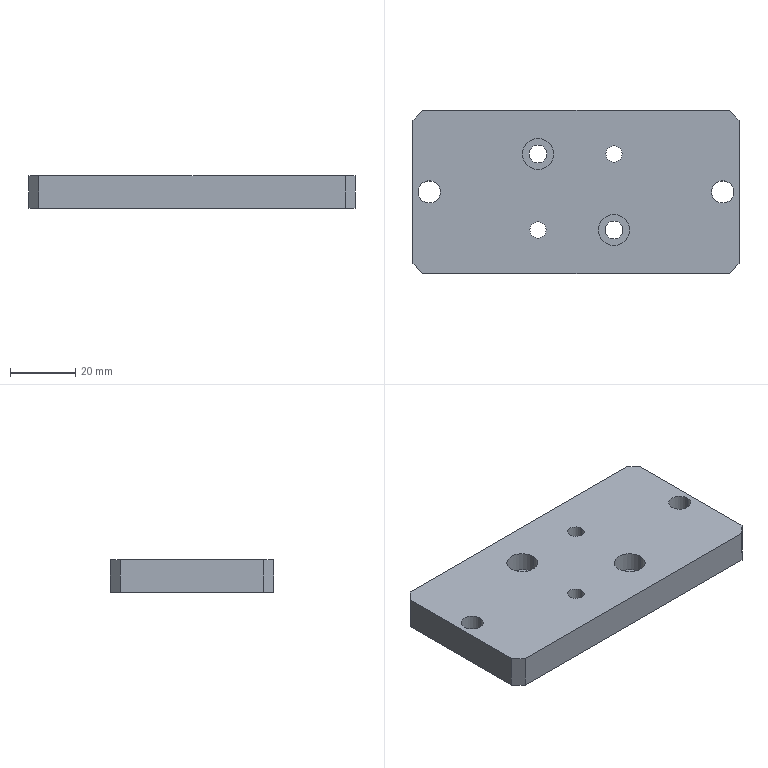Part | STEP file | PN_0002 top plate Default | 1 solid | 28 faces | box 100 x 50 x 10 mm | volume 47660 mm3 | cylinder 16 | plane 12 | commonest cylinder face diameters 5 x4 5.5 x4 6.8 x4 9.5 x4
STEP:
#1=CARTESIAN_POINT('',(-48.4,0.,0.));
#2=VERTEX_POINT('',#1);
#3=CARTESIAN_POINT('',(-41.6,0.,0.));
#4=VERTEX_POINT('',#3);
#5=CARTESIAN_POINT('',(-45.,0.,0.));
#6=DIRECTION('',(0.,0.,1.));
#7=DIRECTION('',(1.,0.,0.));
#8=AXIS2_PLACEMENT_3D('',#5,#6,#7);
#9=CIRCLE('',#8,3.4);
#10=EDGE_CURVE('',#2,#4,#9,.T.);
#11=ORIENTED_EDGE('',*,*,#10,.F.);
#12=CARTESIAN_POINT('',(-48.4,0.,10.));
#13=VERTEX_POINT('',#12);
#14=CARTESIAN_POINT('',(-48.4,0.,10.));
#15=DIRECTION('',(0.,0.,1.));
#16=VECTOR('',#15,1000.);
#17=LINE('',#14,#16);
#18=EDGE_CURVE('',#2,#13,#17,.T.);
#19=ORIENTED_EDGE('',*,*,#18,.T.);
#20=CARTESIAN_POINT('',(-41.6,0.,10.));
#21=VERTEX_POINT('',#20);
#22=CARTESIAN_POINT('',(-45.,0.,10.));
#23=DIRECTION('',(0.,0.,1.));
#24=DIRECTION('',(1.,0.,0.));
#25=AXIS2_PLACEMENT_3D('',#22,#23,#24);
#26=CIRCLE('',#25,3.4);
#27=EDGE_CURVE('',#13,#21,#26,.T.);
#28=ORIENTED_EDGE('',*,*,#27,.T.);
#29=CARTESIAN_POINT('',(-41.6,0.,10.));
#30=DIRECTION('',(0.,0.,1.));
#31=VECTOR('',#30,1000.);
#32=LINE('',#29,#31);
#33=EDGE_CURVE('',#4,#21,#32,.T.);
#34=ORIENTED_EDGE('',*,*,#33,.F.);
#35=EDGE_LOOP('',(#11,#19,#28,#34));
#36=FACE_OUTER_BOUND('',#35,.T.);
#37=CARTESIAN_POINT('',(-45.,0.,10.));
#38=DIRECTION('',(0.,0.,1.));
#39=DIRECTION('',(1.,0.,0.));
#40=AXIS2_PLACEMENT_3D('',#37,#38,#39);
#41=CYLINDRICAL_SURFACE('',#40,3.4);
#42=ADVANCED_FACE('',(#36),#41,.F.);
#43=CARTESIAN_POINT('',(41.6,0.,0.));
#44=VERTEX_POINT('',#43);
#45=CARTESIAN_POINT('',(48.4,0.,0.));
#46=VERTEX_POINT('',#45);
#47=CARTESIAN_POINT('',(45.,0.,0.));
#48=DIRECTION('',(0.,0.,1.));
#49=DIRECTION('',(1.,0.,0.));
#50=AXIS2_PLACEMENT_3D('',#47,#48,#49);
#51=CIRCLE('',#50,3.4);
#52=EDGE_CURVE('',#44,#46,#51,.T.);
#53=ORIENTED_EDGE('',*,*,#52,.F.);
#54=CARTESIAN_POINT('',(41.6,0.,10.));
#55=VERTEX_POINT('',#54);
#56=CARTESIAN_POINT('',(41.6,0.,10.));
#57=DIRECTION('',(0.,0.,1.));
#58=VECTOR('',#57,1000.);
#59=LINE('',#56,#58);
#60=EDGE_CURVE('',#44,#55,#59,.T.);
#61=ORIENTED_EDGE('',*,*,#60,.T.);
#62=CARTESIAN_POINT('',(48.4,0.,10.));
#63=VERTEX_POINT('',#62);
#64=CARTESIAN_POINT('',(45.,0.,10.));
#65=DIRECTION('',(0.,0.,1.));
#66=DIRECTION('',(1.,0.,0.));
#67=AXIS2_PLACEMENT_3D('',#64,#65,#66);
#68=CIRCLE('',#67,3.4);
#69=EDGE_CURVE('',#55,#63,#68,.T.);
#70=ORIENTED_EDGE('',*,*,#69,.T.);
#71=CARTESIAN_POINT('',(48.4,0.,10.));
#72=DIRECTION('',(0.,0.,1.));
#73=VECTOR('',#72,1000.);
#74=LINE('',#71,#73);
#75=EDGE_CURVE('',#46,#63,#74,.T.);
#76=ORIENTED_EDGE('',*,*,#75,.F.);
#77=EDGE_LOOP('',(#53,#61,#70,#76));
#78=FACE_OUTER_BOUND('',#77,.T.);
#79=CARTESIAN_POINT('',(45.,0.,10.));
#80=DIRECTION('',(0.,0.,1.));
#81=DIRECTION('',(1.,0.,0.));
#82=AXIS2_PLACEMENT_3D('',#79,#80,#81);
#83=CYLINDRICAL_SURFACE('',#82,3.4);
#84=ADVANCED_FACE('',(#78),#83,.F.);
#85=CARTESIAN_POINT('',(9.15,11.65,0.));
#86=VERTEX_POINT('',#85);
#87=CARTESIAN_POINT('',(14.15,11.65,0.));
#88=VERTEX_POINT('',#87);
#89=CARTESIAN_POINT('',(11.65,11.65,0.));
#90=DIRECTION('',(0.,0.,1.));
#91=DIRECTION('',(1.,0.,0.));
#92=AXIS2_PLACEMENT_3D('',#89,#90,#91);
#93=CIRCLE('',#92,2.5);
#94=EDGE_CURVE('',#86,#88,#93,.T.);
#95=ORIENTED_EDGE('',*,*,#94,.F.);
#96=CARTESIAN_POINT('',(9.15,11.65,10.));
#97=VERTEX_POINT('',#96);
#98=CARTESIAN_POINT('',(9.15,11.65,10.));
#99=DIRECTION('',(0.,0.,1.));
#100=VECTOR('',#99,1000.);
#101=LINE('',#98,#100);
#102=EDGE_CURVE('',#86,#97,#101,.T.);
#103=ORIENTED_EDGE('',*,*,#102,.T.);
#104=CARTESIAN_POINT('',(14.15,11.65,10.));
#105=VERTEX_POINT('',#104);
#106=CARTESIAN_POINT('',(11.65,11.65,10.));
#107=DIRECTION('',(0.,0.,1.));
#108=DIRECTION('',(1.,0.,0.));
#109=AXIS2_PLACEMENT_3D('',#106,#107,#108);
#110=CIRCLE('',#109,2.5);
#111=EDGE_CURVE('',#97,#105,#110,.T.);
#112=ORIENTED_EDGE('',*,*,#111,.T.);
#113=CARTESIAN_POINT('',(14.15,11.65,10.));
#114=DIRECTION('',(0.,0.,1.));
#115=VECTOR('',#114,1000.);
#116=LINE('',#113,#115);
#117=EDGE_CURVE('',#88,#105,#116,.T.);
#118=ORIENTED_EDGE('',*,*,#117,.F.);
#119=EDGE_LOOP('',(#95,#103,#112,#118));
#120=FACE_OUTER_BOUND('',#119,.T.);
#121=CARTESIAN_POINT('',(11.65,11.65,10.));
#122=DIRECTION('',(0.,0.,1.));
#123=DIRECTION('',(1.,0.,0.));
#124=AXIS2_PLACEMENT_3D('',#121,#122,#123);
#125=CYLINDRICAL_SURFACE('',#124,2.5);
#126=ADVANCED_FACE('',(#120),#125,.F.);
#127=CARTESIAN_POINT('',(-14.15,-11.65,0.));
#128=VERTEX_POINT('',#127);
#129=CARTESIAN_POINT('',(-9.15,-11.65,0.));
#130=VERTEX_POINT('',#129);
#131=CARTESIAN_POINT('',(-11.65,-11.65,0.));
#132=DIRECTION('',(0.,0.,1.));
#133=DIRECTION('',(1.,0.,0.));
#134=AXIS2_PLACEMENT_3D('',#131,#132,#133);
#135=CIRCLE('',#134,2.5);
#136=EDGE_CURVE('',#128,#130,#135,.T.);
#137=ORIENTED_EDGE('',*,*,#136,.F.);
#138=CARTESIAN_POINT('',(-14.15,-11.65,10.));
#139=VERTEX_POINT('',#138);
#140=CARTESIAN_POINT('',(-14.15,-11.65,10.));
#141=DIRECTION('',(0.,0.,1.));
#142=VECTOR('',#141,1000.);
#143=LINE('',#140,#142);
#144=EDGE_CURVE('',#128,#139,#143,.T.);
#145=ORIENTED_EDGE('',*,*,#144,.T.);
#146=CARTESIAN_POINT('',(-9.15,-11.65,10.));
#147=VERTEX_POINT('',#146);
#148=CARTESIAN_POINT('',(-11.65,-11.65,10.));
#149=DIRECTION('',(0.,0.,1.));
#150=DIRECTION('',(1.,0.,0.));
#151=AXIS2_PLACEMENT_3D('',#148,#149,#150);
#152=CIRCLE('',#151,2.5);
#153=EDGE_CURVE('',#139,#147,#152,.T.);
#154=ORIENTED_EDGE('',*,*,#153,.T.);
#155=CARTESIAN_POINT('',(-9.15,-11.65,10.));
#156=DIRECTION('',(0.,0.,1.));
#157=VECTOR('',#156,1000.);
#158=LINE('',#155,#157);
#159=EDGE_CURVE('',#130,#147,#158,.T.);
#160=ORIENTED_EDGE('',*,*,#159,.F.);
#161=EDGE_LOOP('',(#137,#145,#154,#160));
#162=FACE_OUTER_BOUND('',#161,.T.);
#163=CARTESIAN_POINT('',(-11.65,-11.65,10.));
#164=DIRECTION('',(0.,0.,1.));
#165=DIRECTION('',(1.,0.,0.));
#166=AXIS2_PLACEMENT_3D('',#163,#164,#165);
#167=CYLINDRICAL_SURFACE('',#166,2.5);
#168=ADVANCED_FACE('',(#162),#167,.F.);
#169=CARTESIAN_POINT('',(6.9,-11.65,4.));
#170=VERTEX_POINT('',#169);
#171=CARTESIAN_POINT('',(16.4,-11.65,4.));
#172=VERTEX_POINT('',#171);
#173=CARTESIAN_POINT('',(11.65,-11.65,4.));
#174=DIRECTION('',(0.,0.,1.));
#175=DIRECTION('',(1.,0.,0.));
#176=AXIS2_PLACEMENT_3D('',#173,#174,#175);
#177=CIRCLE('',#176,4.75);
#178=EDGE_CURVE('',#170,#172,#177,.T.);
#179=ORIENTED_EDGE('',*,*,#178,.F.);
#180=CARTESIAN_POINT('',(6.9,-11.65,10.));
#181=VERTEX_POINT('',#180);
#182=CARTESIAN_POINT('',(6.9,-11.65,10.));
#183=DIRECTION('',(0.,0.,1.));
#184=VECTOR('',#183,1000.);
#185=LINE('',#182,#184);
#186=EDGE_CURVE('',#170,#181,#185,.T.);
#187=ORIENTED_EDGE('',*,*,#186,.T.);
#188=CARTESIAN_POINT('',(16.4,-11.65,10.));
#189=VERTEX_POINT('',#188);
#190=CARTESIAN_POINT('',(11.65,-11.65,10.));
#191=DIRECTION('',(0.,0.,1.));
#192=DIRECTION('',(1.,0.,0.));
#193=AXIS2_PLACEMENT_3D('',#190,#191,#192);
#194=CIRCLE('',#193,4.75);
#195=EDGE_CURVE('',#181,#189,#194,.T.);
#196=ORIENTED_EDGE('',*,*,#195,.T.);
#197=CARTESIAN_POINT('',(16.4,-11.65,10.));
#198=DIRECTION('',(0.,0.,1.));
#199=VECTOR('',#198,1000.);
#200=LINE('',#197,#199);
#201=EDGE_CURVE('',#172,#189,#200,.T.);
#202=ORIENTED_EDGE('',*,*,#201,.F.);
#203=EDGE_LOOP('',(#179,#187,#196,#202));
#204=FACE_OUTER_BOUND('',#203,.T.);
#205=CARTESIAN_POINT('',(11.65,-11.65,10.));
#206=DIRECTION('',(0.,0.,1.));
#207=DIRECTION('',(1.,0.,0.));
#208=AXIS2_PLACEMENT_3D('',#205,#206,#207);
#209=CYLINDRICAL_SURFACE('',#208,4.75);
#210=ADVANCED_FACE('',(#204),#209,.F.);
#211=CARTESIAN_POINT('',(8.9,-11.65,0.));
#212=VERTEX_POINT('',#211);
#213=CARTESIAN_POINT('',(14.4,-11.65,0.));
#214=VERTEX_POINT('',#213);
#215=CARTESIAN_POINT('',(11.65,-11.65,0.));
#216=DIRECTION('',(0.,0.,1.));
#217=DIRECTION('',(1.,0.,0.));
#218=AXIS2_PLACEMENT_3D('',#215,#216,#217);
#219=CIRCLE('',#218,2.75);
#220=EDGE_CURVE('',#212,#214,#219,.T.);
#221=ORIENTED_EDGE('',*,*,#220,.F.);
#222=CARTESIAN_POINT('',(8.9,-11.65,4.));
#223=VERTEX_POINT('',#222);
#224=CARTESIAN_POINT('',(8.9,-11.65,10.));
#225=DIRECTION('',(0.,0.,1.));
#226=VECTOR('',#225,1000.);
#227=LINE('',#224,#226);
#228=EDGE_CURVE('',#212,#223,#227,.T.);
#229=ORIENTED_EDGE('',*,*,#228,.T.);
#230=CARTESIAN_POINT('',(14.4,-11.65,4.));
#231=VERTEX_POINT('',#230);
#232=CARTESIAN_POINT('',(11.65,-11.65,4.));
#233=DIRECTION('',(0.,0.,1.));
#234=DIRECTION('',(1.,0.,0.));
#235=AXIS2_PLACEMENT_3D('',#232,#233,#234);
#236=CIRCLE('',#235,2.75);
#237=EDGE_CURVE('',#223,#231,#236,.T.);
#238=ORIENTED_EDGE('',*,*,#237,.T.);
#239=CARTESIAN_POINT('',(14.4,-11.65,10.));
#240=DIRECTION('',(0.,0.,1.));
#241=VECTOR('',#240,1000.);
#242=LINE('',#239,#241);
#243=EDGE_CURVE('',#214,#231,#242,.T.);
#244=ORIENTED_EDGE('',*,*,#243,.F.);
#245=EDGE_LOOP('',(#221,#229,#238,#244));
#246=FACE_OUTER_BOUND('',#245,.T.);
#247=CARTESIAN_POINT('',(11.65,-11.65,10.));
#248=DIRECTION('',(0.,0.,1.));
#249=DIRECTION('',(1.,0.,0.));
#250=AXIS2_PLACEMENT_3D('',#247,#248,#249);
#251=CYLINDRICAL_SURFACE('',#250,2.75);
#252=ADVANCED_FACE('',(#246),#251,.F.);
#253=CARTESIAN_POINT('',(-16.4,11.65,4.));
#254=VERTEX_POINT('',#253);
#255=CARTESIAN_POINT('',(-6.9,11.65,4.));
#256=VERTEX_POINT('',#255);
#257=CARTESIAN_POINT('',(-11.65,11.65,4.));
#258=DIRECTION('',(0.,0.,1.));
#259=DIRECTION('',(1.,0.,0.));
#260=AXIS2_PLACEMENT_3D('',#257,#258,#259);
#261=CIRCLE('',#260,4.75);
#262=EDGE_CURVE('',#254,#256,#261,.T.);
#263=ORIENTED_EDGE('',*,*,#262,.F.);
#264=CARTESIAN_POINT('',(-16.4,11.65,10.));
#265=VERTEX_POINT('',#264);
#266=CARTESIAN_POINT('',(-16.4,11.65,10.));
#267=DIRECTION('',(0.,0.,1.));
#268=VECTOR('',#267,1000.);
#269=LINE('',#266,#268);
#270=EDGE_CURVE('',#254,#265,#269,.T.);
#271=ORIENTED_EDGE('',*,*,#270,.T.);
#272=CARTESIAN_POINT('',(-6.9,11.65,10.));
#273=VERTEX_POINT('',#272);
#274=CARTESIAN_POINT('',(-11.65,11.65,10.));
#275=DIRECTION('',(0.,0.,1.));
#276=DIRECTION('',(1.,0.,0.));
#277=AXIS2_PLACEMENT_3D('',#274,#275,#276);
#278=CIRCLE('',#277,4.75);
#279=EDGE_CURVE('',#265,#273,#278,.T.);
#280=ORIENTED_EDGE('',*,*,#279,.T.);
#281=CARTESIAN_POINT('',(-6.9,11.65,10.));
#282=DIRECTION('',(0.,0.,1.));
#283=VECTOR('',#282,1000.);
#284=LINE('',#281,#283);
#285=EDGE_CURVE('',#256,#273,#284,.T.);
#286=ORIENTED_EDGE('',*,*,#285,.F.);
#287=EDGE_LOOP('',(#263,#271,#280,#286));
#288=FACE_OUTER_BOUND('',#287,.T.);
#289=CARTESIAN_POINT('',(-11.65,11.65,10.));
#290=DIRECTION('',(0.,0.,1.));
#291=DIRECTION('',(1.,0.,0.));
#292=AXIS2_PLACEMENT_3D('',#289,#290,#291);
#293=CYLINDRICAL_SURFACE('',#292,4.75);
#294=ADVANCED_FACE('',(#288),#293,.F.);
#295=CARTESIAN_POINT('',(-14.4,11.65,0.));
#296=VERTEX_POINT('',#295);
#297=CARTESIAN_POINT('',(-8.9,11.65,0.));
#298=VERTEX_POINT('',#297);
#299=CARTESIAN_POINT('',(-11.65,11.65,0.));
#300=DIRECTION('',(0.,0.,1.));
#301=DIRECTION('',(1.,0.,0.));
#302=AXIS2_PLACEMENT_3D('',#299,#300,#301);
#303=CIRCLE('',#302,2.75);
#304=EDGE_CURVE('',#296,#298,#303,.T.);
#305=ORIENTED_EDGE('',*,*,#304,.F.);
#306=CARTESIAN_POINT('',(-14.4,11.65,4.));
#307=VERTEX_POINT('',#306);
#308=CARTESIAN_POINT('',(-14.4,11.65,10.));
#309=DIRECTION('',(0.,0.,1.));
#310=VECTOR('',#309,1000.);
#311=LINE('',#308,#310);
#312=EDGE_CURVE('',#296,#307,#311,.T.);
#313=ORIENTED_EDGE('',*,*,#312,.T.);
#314=CARTESIAN_POINT('',(-8.9,11.65,4.));
#315=VERTEX_POINT('',#314);
#316=CARTESIAN_POINT('',(-11.65,11.65,4.));
#317=DIRECTION('',(0.,0.,1.));
#318=DIRECTION('',(1.,0.,0.));
#319=AXIS2_PLACEMENT_3D('',#316,#317,#318);
#320=CIRCLE('',#319,2.75);
#321=EDGE_CURVE('',#307,#315,#320,.T.);
#322=ORIENTED_EDGE('',*,*,#321,.T.);
#323=CARTESIAN_POINT('',(-8.9,11.65,10.));
#324=DIRECTION('',(0.,0.,1.));
#325=VECTOR('',#324,1000.);
#326=LINE('',#323,#325);
#327=EDGE_CURVE('',#298,#315,#326,.T.);
#328=ORIENTED_EDGE('',*,*,#327,.F.);
#329=EDGE_LOOP('',(#305,#313,#322,#328));
#330=FACE_OUTER_BOUND('',#329,.T.);
#331=CARTESIAN_POINT('',(-11.65,11.65,10.));
#332=DIRECTION('',(0.,0.,1.));
#333=DIRECTION('',(1.,0.,0.));
#334=AXIS2_PLACEMENT_3D('',#331,#332,#333);
#335=CYLINDRICAL_SURFACE('',#334,2.75);
#336=ADVANCED_FACE('',(#330),#335,.F.);
#337=CARTESIAN_POINT('',(50.,-22.,0.));
#338=VERTEX_POINT('',#337);
#339=CARTESIAN_POINT('',(50.,22.,0.));
#340=VERTEX_POINT('',#339);
#341=CARTESIAN_POINT('',(50.,25.,0.));
#342=DIRECTION('',(0.,1.,0.));
#343=VECTOR('',#342,1000.);
#344=LINE('',#341,#343);
#345=EDGE_CURVE('',#338,#340,#344,.T.);
#346=ORIENTED_EDGE('',*,*,#345,.T.);
#347=CARTESIAN_POINT('',(50.,22.,10.));
#348=VERTEX_POINT('',#347);
#349=CARTESIAN_POINT('',(50.,22.,10.));
#350=DIRECTION('',(0.,0.,1.));
#351=VECTOR('',#350,1000.);
#352=LINE('',#349,#351);
#353=EDGE_CURVE('',#340,#348,#352,.T.);
#354=ORIENTED_EDGE('',*,*,#353,.T.);
#355=CARTESIAN_POINT('',(50.,-22.,10.));
#356=VERTEX_POINT('',#355);
#357=CARTESIAN_POINT('',(50.,25.,10.));
#358=DIRECTION('',(0.,1.,0.));
#359=VECTOR('',#358,1000.);
#360=LINE('',#357,#359);
#361=EDGE_CURVE('',#356,#348,#360,.T.);
#362=ORIENTED_EDGE('',*,*,#361,.F.);
#363=CARTESIAN_POINT('',(50.,-22.,10.));
#364=DIRECTION('',(0.,0.,-1.));
#365=VECTOR('',#364,1000.);
#366=LINE('',#363,#365);
#367=EDGE_CURVE('',#356,#338,#366,.T.);
#368=ORIENTED_EDGE('',*,*,#367,.T.);
#369=EDGE_LOOP('',(#346,#354,#362,#368));
#370=FACE_OUTER_BOUND('',#369,.T.);
#371=CARTESIAN_POINT('',(50.,25.,10.));
#372=DIRECTION('',(-1.,0.,0.));
#373=DIRECTION('',(0.,-1.,0.));
#374=AXIS2_PLACEMENT_3D('',#371,#372,#373);
#375=PLANE('',#374);
#376=ADVANCED_FACE('',(#370),#375,.F.);
#377=CARTESIAN_POINT('',(47.,25.,0.));
#378=VERTEX_POINT('',#377);
#379=CARTESIAN_POINT('',(-47.,25.,0.));
#380=VERTEX_POINT('',#379);
#381=CARTESIAN_POINT('',(-50.,25.,0.));
#382=DIRECTION('',(-1.,0.,0.));
#383=VECTOR('',#382,1000.);
#384=LINE('',#381,#383);
#385=EDGE_CURVE('',#378,#380,#384,.T.);
#386=ORIENTED_EDGE('',*,*,#385,.T.);
#387=CARTESIAN_POINT('',(-47.,25.,10.));
#388=VERTEX_POINT('',#387);
#389=CARTESIAN_POINT('',(-47.,25.,10.));
#390=DIRECTION('',(0.,0.,1.));
#391=VECTOR('',#390,1000.);
#392=LINE('',#389,#391);
#393=EDGE_CURVE('',#380,#388,#392,.T.);
#394=ORIENTED_EDGE('',*,*,#393,.T.);
#395=CARTESIAN_POINT('',(47.,25.,10.));
#396=VERTEX_POINT('',#395);
#397=CARTESIAN_POINT('',(-50.,25.,10.));
#398=DIRECTION('',(-1.,0.,0.));
#399=VECTOR('',#398,1000.);
#400=LINE('',#397,#399);
#401=EDGE_CURVE('',#396,#388,#400,.T.);
#402=ORIENTED_EDGE('',*,*,#401,.F.);
#403=CARTESIAN_POINT('',(47.,25.,10.));
#404=DIRECTION('',(0.,0.,-1.));
#405=VECTOR('',#404,1000.);
#406=LINE('',#403,#405);
#407=EDGE_CURVE('',#396,#378,#406,.T.);
#408=ORIENTED_EDGE('',*,*,#407,.T.);
#409=EDGE_LOOP('',(#386,#394,#402,#408));
#410=FACE_OUTER_BOUND('',#409,.T.);
#411=CARTESIAN_POINT('',(-50.,25.,10.));
#412=DIRECTION('',(0.,-1.,0.));
#413=DIRECTION('',(0.,0.,-1.));
#414=AXIS2_PLACEMENT_3D('',#411,#412,#413);
#415=PLANE('',#414);
#416=ADVANCED_FACE('',(#410),#415,.F.);
#417=CARTESIAN_POINT('',(-50.,22.,10.));
#418=VERTEX_POINT('',#417);
#419=CARTESIAN_POINT('',(-50.,-22.,10.));
#420=VERTEX_POINT('',#419);
#421=CARTESIAN_POINT('',(-50.,25.,10.));
#422=DIRECTION('',(0.,-1.,0.));
#423=VECTOR('',#422,1000.);
#424=LINE('',#421,#423);
#425=EDGE_CURVE('',#418,#420,#424,.T.);
#426=ORIENTED_EDGE('',*,*,#425,.F.);
#427=CARTESIAN_POINT('',(-50.,22.,0.));
#428=VERTEX_POINT('',#427);
#429=CARTESIAN_POINT('',(-50.,22.,10.));
#430=DIRECTION('',(0.,0.,-1.));
#431=VECTOR('',#430,1000.);
#432=LINE('',#429,#431);
#433=EDGE_CURVE('',#418,#428,#432,.T.);
#434=ORIENTED_EDGE('',*,*,#433,.T.);
#435=CARTESIAN_POINT('',(-50.,-22.,0.));
#436=VERTEX_POINT('',#435);
#437=CARTESIAN_POINT('',(-50.,25.,0.));
#438=DIRECTION('',(0.,-1.,0.));
#439=VECTOR('',#438,1000.);
#440=LINE('',#437,#439);
#441=EDGE_CURVE('',#428,#436,#440,.T.);
#442=ORIENTED_EDGE('',*,*,#441,.T.);
#443=CARTESIAN_POINT('',(-50.,-22.,10.));
#444=DIRECTION('',(0.,0.,1.));
#445=VECTOR('',#444,1000.);
#446=LINE('',#443,#445);
#447=EDGE_CURVE('',#436,#420,#446,.T.);
#448=ORIENTED_EDGE('',*,*,#447,.T.);
#449=EDGE_LOOP('',(#426,#434,#442,#448));
#450=FACE_OUTER_BOUND('',#449,.T.);
#451=CARTESIAN_POINT('',(-50.,25.,10.));
#452=DIRECTION('',(1.,0.,0.));
#453=DIRECTION('',(0.,1.,0.));
#454=AXIS2_PLACEMENT_3D('',#451,#452,#453);
#455=PLANE('',#454);
#456=ADVANCED_FACE('',(#450),#455,.F.);
#457=CARTESIAN_POINT('',(-47.,-25.,0.));
#458=VERTEX_POINT('',#457);
#459=CARTESIAN_POINT('',(47.,-25.,0.));
#460=VERTEX_POINT('',#459);
#461=CARTESIAN_POINT('',(-50.,-25.,0.));
#462=DIRECTION('',(1.,0.,0.));
#463=VECTOR('',#462,1000.);
#464=LINE('',#461,#463);
#465=EDGE_CURVE('',#458,#460,#464,.T.);
#466=ORIENTED_EDGE('',*,*,#465,.T.);
#467=CARTESIAN_POINT('',(47.,-25.,10.));
#468=VERTEX_POINT('',#467);
#469=CARTESIAN_POINT('',(47.,-25.,10.));
#470=DIRECTION('',(0.,0.,1.));
#471=VECTOR('',#470,1000.);
#472=LINE('',#469,#471);
#473=EDGE_CURVE('',#460,#468,#472,.T.);
#474=ORIENTED_EDGE('',*,*,#473,.T.);
#475=CARTESIAN_POINT('',(-47.,-25.,10.));
#476=VERTEX_POINT('',#475);
#477=CARTESIAN_POINT('',(-50.,-25.,10.));
#478=DIRECTION('',(1.,0.,0.));
#479=VECTOR('',#478,1000.);
#480=LINE('',#477,#479);
#481=EDGE_CURVE('',#476,#468,#480,.T.);
#482=ORIENTED_EDGE('',*,*,#481,.F.);
#483=CARTESIAN_POINT('',(-47.,-25.,10.));
#484=DIRECTION('',(0.,0.,-1.));
#485=VECTOR('',#484,1000.);
#486=LINE('',#483,#485);
#487=EDGE_CURVE('',#476,#458,#486,.T.);
#488=ORIENTED_EDGE('',*,*,#487,.T.);
#489=EDGE_LOOP('',(#466,#474,#482,#488));
#490=FACE_OUTER_BOUND('',#489,.T.);
#491=CARTESIAN_POINT('',(-50.,-25.,10.));
#492=DIRECTION('',(0.,1.,0.));
#493=DIRECTION('',(0.,0.,1.));
#494=AXIS2_PLACEMENT_3D('',#491,#492,#493);
#495=PLANE('',#494);
#496=ADVANCED_FACE('',(#490),#495,.F.);
#497=CARTESIAN_POINT('',(-45.,0.,10.));
#498=DIRECTION('',(0.,0.,1.));
#499=DIRECTION('',(1.,0.,0.));
#500=AXIS2_PLACEMENT_3D('',#497,#498,#499);
#501=CIRCLE('',#500,3.4);
#502=EDGE_CURVE('',#21,#13,#501,.T.);
#503=ORIENTED_EDGE('',*,*,#502,.F.);
#504=ORIENTED_EDGE('',*,*,#27,.F.);
#505=EDGE_LOOP('',(#503,#504));
#506=FACE_BOUND('',#505,.T.);
#507=CARTESIAN_POINT('',(45.,0.,10.));
#508=DIRECTION('',(0.,0.,1.));
#509=DIRECTION('',(1.,0.,0.));
#510=AXIS2_PLACEMENT_3D('',#507,#508,#509);
#511=CIRCLE('',#510,3.4);
#512=EDGE_CURVE('',#63,#55,#511,.T.);
#513=ORIENTED_EDGE('',*,*,#512,.F.);
#514=ORIENTED_EDGE('',*,*,#69,.F.);
#515=EDGE_LOOP('',(#513,#514));
#516=FACE_BOUND('',#515,.T.);
#517=CARTESIAN_POINT('',(11.65,11.65,10.));
#518=DIRECTION('',(0.,0.,1.));
#519=DIRECTION('',(1.,0.,0.));
#520=AXIS2_PLACEMENT_3D('',#517,#518,#519);
#521=CIRCLE('',#520,2.5);
#522=EDGE_CURVE('',#105,#97,#521,.T.);
#523=ORIENTED_EDGE('',*,*,#522,.F.);
#524=ORIENTED_EDGE('',*,*,#111,.F.);
#525=EDGE_LOOP('',(#523,#524));
#526=FACE_BOUND('',#525,.T.);
#527=CARTESIAN_POINT('',(-11.65,-11.65,10.));
#528=DIRECTION('',(0.,0.,1.));
#529=DIRECTION('',(1.,0.,0.));
#530=AXIS2_PLACEMENT_3D('',#527,#528,#529);
#531=CIRCLE('',#530,2.5);
#532=EDGE_CURVE('',#147,#139,#531,.T.);
#533=ORIENTED_EDGE('',*,*,#532,.F.);
#534=ORIENTED_EDGE('',*,*,#153,.F.);
#535=EDGE_LOOP('',(#533,#534));
#536=FACE_BOUND('',#535,.T.);
#537=CARTESIAN_POINT('',(11.65,-11.65,10.));
#538=DIRECTION('',(0.,0.,1.));
#539=DIRECTION('',(1.,0.,0.));
#540=AXIS2_PLACEMENT_3D('',#537,#538,#539);
#541=CIRCLE('',#540,4.75);
#542=EDGE_CURVE('',#189,#181,#541,.T.);
#543=ORIENTED_EDGE('',*,*,#542,.F.);
#544=ORIENTED_EDGE('',*,*,#195,.F.);
#545=EDGE_LOOP('',(#543,#544));
#546=FACE_BOUND('',#545,.T.);
#547=CARTESIAN_POINT('',(-11.65,11.65,10.));
#548=DIRECTION('',(0.,0.,1.));
#549=DIRECTION('',(1.,0.,0.));
#550=AXIS2_PLACEMENT_3D('',#547,#548,#549);
#551=CIRCLE('',#550,4.75);
#552=EDGE_CURVE('',#273,#265,#551,.T.);
#553=ORIENTED_EDGE('',*,*,#552,.F.);
#554=ORIENTED_EDGE('',*,*,#279,.F.);
#555=EDGE_LOOP('',(#553,#554));
#556=FACE_BOUND('',#555,.T.);
#557=ORIENTED_EDGE('',*,*,#401,.T.);
#558=CARTESIAN_POINT('',(-36.,36.,10.));
#559=DIRECTION('',(-0.7071,-0.7071,0.));
#560=VECTOR('',#559,1000.);
#561=LINE('',#558,#560);
#562=EDGE_CURVE('',#388,#418,#561,.T.);
#563=ORIENTED_EDGE('',*,*,#562,.T.);
#564=ORIENTED_EDGE('',*,*,#425,.T.);
#565=CARTESIAN_POINT('',(-36.,-36.,10.));
#566=DIRECTION('',(0.7071,-0.7071,0.));
#567=VECTOR('',#566,1000.);
#568=LINE('',#565,#567);
#569=EDGE_CURVE('',#420,#476,#568,.T.);
#570=ORIENTED_EDGE('',*,*,#569,.T.);
#571=ORIENTED_EDGE('',*,*,#481,.T.);
#572=CARTESIAN_POINT('',(36.,-36.,10.));
#573=DIRECTION('',(0.7071,0.7071,0.));
#574=VECTOR('',#573,1000.);
#575=LINE('',#572,#574);
#576=EDGE_CURVE('',#468,#356,#575,.T.);
#577=ORIENTED_EDGE('',*,*,#576,.T.);
#578=ORIENTED_EDGE('',*,*,#361,.T.);
#579=CARTESIAN_POINT('',(36.,36.,10.));
#580=DIRECTION('',(-0.7071,0.7071,0.));
#581=VECTOR('',#580,1000.);
#582=LINE('',#579,#581);
#583=EDGE_CURVE('',#348,#396,#582,.T.);
#584=ORIENTED_EDGE('',*,*,#583,.T.);
#585=EDGE_LOOP('',(#557,#563,#564,#570,#571,#577,#578,#584));
#586=FACE_OUTER_BOUND('',#585,.T.);
#587=CARTESIAN_POINT('',(0.,0.,10.));
#588=DIRECTION('',(0.,0.,1.));
#589=DIRECTION('',(1.,0.,0.));
#590=AXIS2_PLACEMENT_3D('',#587,#588,#589);
#591=PLANE('',#590);
#592=ADVANCED_FACE('',(#506,#516,#526,#536,#546,#556,#586),#591,.T.);
#593=CARTESIAN_POINT('',(-45.,0.,0.));
#594=DIRECTION('',(0.,0.,1.));
#595=DIRECTION('',(1.,0.,0.));
#596=AXIS2_PLACEMENT_3D('',#593,#594,#595);
#597=CIRCLE('',#596,3.4);
#598=EDGE_CURVE('',#4,#2,#597,.T.);
#599=ORIENTED_EDGE('',*,*,#598,.T.);
#600=ORIENTED_EDGE('',*,*,#10,.T.);
#601=EDGE_LOOP('',(#599,#600));
#602=FACE_BOUND('',#601,.T.);
#603=CARTESIAN_POINT('',(45.,0.,0.));
#604=DIRECTION('',(0.,0.,1.));
#605=DIRECTION('',(1.,0.,0.));
#606=AXIS2_PLACEMENT_3D('',#603,#604,#605);
#607=CIRCLE('',#606,3.4);
#608=EDGE_CURVE('',#46,#44,#607,.T.);
#609=ORIENTED_EDGE('',*,*,#608,.T.);
#610=ORIENTED_EDGE('',*,*,#52,.T.);
#611=EDGE_LOOP('',(#609,#610));
#612=FACE_BOUND('',#611,.T.);
#613=CARTESIAN_POINT('',(11.65,11.65,0.));
#614=DIRECTION('',(0.,0.,1.));
#615=DIRECTION('',(1.,0.,0.));
#616=AXIS2_PLACEMENT_3D('',#613,#614,#615);
#617=CIRCLE('',#616,2.5);
#618=EDGE_CURVE('',#88,#86,#617,.T.);
#619=ORIENTED_EDGE('',*,*,#618,.T.);
#620=ORIENTED_EDGE('',*,*,#94,.T.);
#621=EDGE_LOOP('',(#619,#620));
#622=FACE_BOUND('',#621,.T.);
#623=CARTESIAN_POINT('',(-11.65,-11.65,0.));
#624=DIRECTION('',(0.,0.,1.));
#625=DIRECTION('',(1.,0.,0.));
#626=AXIS2_PLACEMENT_3D('',#623,#624,#625);
#627=CIRCLE('',#626,2.5);
#628=EDGE_CURVE('',#130,#128,#627,.T.);
#629=ORIENTED_EDGE('',*,*,#628,.T.);
#630=ORIENTED_EDGE('',*,*,#136,.T.);
#631=EDGE_LOOP('',(#629,#630));
#632=FACE_BOUND('',#631,.T.);
#633=CARTESIAN_POINT('',(11.65,-11.65,0.));
#634=DIRECTION('',(0.,0.,1.));
#635=DIRECTION('',(1.,0.,0.));
#636=AXIS2_PLACEMENT_3D('',#633,#634,#635);
#637=CIRCLE('',#636,2.75);
#638=EDGE_CURVE('',#214,#212,#637,.T.);
#639=ORIENTED_EDGE('',*,*,#638,.T.);
#640=ORIENTED_EDGE('',*,*,#220,.T.);
#641=EDGE_LOOP('',(#639,#640));
#642=FACE_BOUND('',#641,.T.);
#643=CARTESIAN_POINT('',(-11.65,11.65,0.));
#644=DIRECTION('',(0.,0.,1.));
#645=DIRECTION('',(1.,0.,0.));
#646=AXIS2_PLACEMENT_3D('',#643,#644,#645);
#647=CIRCLE('',#646,2.75);
#648=EDGE_CURVE('',#298,#296,#647,.T.);
#649=ORIENTED_EDGE('',*,*,#648,.T.);
#650=ORIENTED_EDGE('',*,*,#304,.T.);
#651=EDGE_LOOP('',(#649,#650));
#652=FACE_BOUND('',#651,.T.);
#653=ORIENTED_EDGE('',*,*,#441,.F.);
#654=CARTESIAN_POINT('',(-50.,22.,0.));
#655=DIRECTION('',(0.7071,0.7071,0.));
#656=VECTOR('',#655,1000.);
#657=LINE('',#654,#656);
#658=EDGE_CURVE('',#428,#380,#657,.T.);
#659=ORIENTED_EDGE('',*,*,#658,.T.);
#660=ORIENTED_EDGE('',*,*,#385,.F.);
#661=CARTESIAN_POINT('',(47.,25.,0.));
#662=DIRECTION('',(0.7071,-0.7071,0.));
#663=VECTOR('',#662,1000.);
#664=LINE('',#661,#663);
#665=EDGE_CURVE('',#378,#340,#664,.T.);
#666=ORIENTED_EDGE('',*,*,#665,.T.);
#667=ORIENTED_EDGE('',*,*,#345,.F.);
#668=CARTESIAN_POINT('',(50.,-22.,0.));
#669=DIRECTION('',(-0.7071,-0.7071,0.));
#670=VECTOR('',#669,1000.);
#671=LINE('',#668,#670);
#672=EDGE_CURVE('',#338,#460,#671,.T.);
#673=ORIENTED_EDGE('',*,*,#672,.T.);
#674=ORIENTED_EDGE('',*,*,#465,.F.);
#675=CARTESIAN_POINT('',(-47.,-25.,0.));
#676=DIRECTION('',(-0.7071,0.7071,0.));
#677=VECTOR('',#676,1000.);
#678=LINE('',#675,#677);
#679=EDGE_CURVE('',#458,#436,#678,.T.);
#680=ORIENTED_EDGE('',*,*,#679,.T.);
#681=EDGE_LOOP('',(#653,#659,#660,#666,#667,#673,#674,#680));
#682=FACE_OUTER_BOUND('',#681,.T.);
#683=CARTESIAN_POINT('',(0.,0.,0.));
#684=DIRECTION('',(0.,0.,1.));
#685=DIRECTION('',(1.,0.,0.));
#686=AXIS2_PLACEMENT_3D('',#683,#684,#685);
#687=PLANE('',#686);
#688=ADVANCED_FACE('',(#602,#612,#622,#632,#642,#652,#682),#687,.F.);
#689=ORIENTED_EDGE('',*,*,#562,.F.);
#690=ORIENTED_EDGE('',*,*,#393,.F.);
#691=ORIENTED_EDGE('',*,*,#658,.F.);
#692=ORIENTED_EDGE('',*,*,#433,.F.);
#693=EDGE_LOOP('',(#689,#690,#691,#692));
#694=FACE_OUTER_BOUND('',#693,.T.);
#695=CARTESIAN_POINT('',(-50.,22.,10.));
#696=DIRECTION('',(0.7071,-0.7071,0.));
#697=DIRECTION('',(0.,0.,-1.));
#698=AXIS2_PLACEMENT_3D('',#695,#696,#697);
#699=PLANE('',#698);
#700=ADVANCED_FACE('',(#694),#699,.F.);
#701=ORIENTED_EDGE('',*,*,#583,.F.);
#702=ORIENTED_EDGE('',*,*,#353,.F.);
#703=ORIENTED_EDGE('',*,*,#665,.F.);
#704=ORIENTED_EDGE('',*,*,#407,.F.);
#705=EDGE_LOOP('',(#701,#702,#703,#704));
#706=FACE_OUTER_BOUND('',#705,.T.);
#707=CARTESIAN_POINT('',(47.,25.,10.));
#708=DIRECTION('',(-0.7071,-0.7071,0.));
#709=DIRECTION('',(0.,0.,-1.));
#710=AXIS2_PLACEMENT_3D('',#707,#708,#709);
#711=PLANE('',#710);
#712=ADVANCED_FACE('',(#706),#711,.F.);
#713=ORIENTED_EDGE('',*,*,#576,.F.);
#714=ORIENTED_EDGE('',*,*,#473,.F.);
#715=ORIENTED_EDGE('',*,*,#672,.F.);
#716=ORIENTED_EDGE('',*,*,#367,.F.);
#717=EDGE_LOOP('',(#713,#714,#715,#716));
#718=FACE_OUTER_BOUND('',#717,.T.);
#719=CARTESIAN_POINT('',(50.,-22.,10.));
#720=DIRECTION('',(-0.7071,0.7071,0.));
#721=DIRECTION('',(0.,0.,-1.));
#722=AXIS2_PLACEMENT_3D('',#719,#720,#721);
#723=PLANE('',#722);
#724=ADVANCED_FACE('',(#718),#723,.F.);
#725=ORIENTED_EDGE('',*,*,#569,.F.);
#726=ORIENTED_EDGE('',*,*,#447,.F.);
#727=ORIENTED_EDGE('',*,*,#679,.F.);
#728=ORIENTED_EDGE('',*,*,#487,.F.);
#729=EDGE_LOOP('',(#725,#726,#727,#728));
#730=FACE_OUTER_BOUND('',#729,.T.);
#731=CARTESIAN_POINT('',(-47.,-25.,10.));
#732=DIRECTION('',(0.7071,0.7071,0.));
#733=DIRECTION('',(0.,0.,-1.));
#734=AXIS2_PLACEMENT_3D('',#731,#732,#733);
#735=PLANE('',#734);
#736=ADVANCED_FACE('',(#730),#735,.F.);
#737=ORIENTED_EDGE('',*,*,#312,.F.);
#738=ORIENTED_EDGE('',*,*,#648,.F.);
#739=ORIENTED_EDGE('',*,*,#327,.T.);
#740=CARTESIAN_POINT('',(-11.65,11.65,4.));
#741=DIRECTION('',(0.,0.,1.));
#742=DIRECTION('',(1.,0.,0.));
#743=AXIS2_PLACEMENT_3D('',#740,#741,#742);
#744=CIRCLE('',#743,2.75);
#745=EDGE_CURVE('',#315,#307,#744,.T.);
#746=ORIENTED_EDGE('',*,*,#745,.T.);
#747=EDGE_LOOP('',(#737,#738,#739,#746));
#748=FACE_OUTER_BOUND('',#747,.T.);
#749=CARTESIAN_POINT('',(-11.65,11.65,10.));
#750=DIRECTION('',(0.,0.,1.));
#751=DIRECTION('',(1.,0.,0.));
#752=AXIS2_PLACEMENT_3D('',#749,#750,#751);
#753=CYLINDRICAL_SURFACE('',#752,2.75);
#754=ADVANCED_FACE('',(#748),#753,.F.);
#755=ORIENTED_EDGE('',*,*,#745,.F.);
#756=ORIENTED_EDGE('',*,*,#321,.F.);
#757=EDGE_LOOP('',(#755,#756));
#758=FACE_BOUND('',#757,.T.);
#759=CARTESIAN_POINT('',(-11.65,11.65,4.));
#760=DIRECTION('',(0.,0.,1.));
#761=DIRECTION('',(1.,0.,0.));
#762=AXIS2_PLACEMENT_3D('',#759,#760,#761);
#763=CIRCLE('',#762,4.75);
#764=EDGE_CURVE('',#256,#254,#763,.T.);
#765=ORIENTED_EDGE('',*,*,#764,.T.);
#766=ORIENTED_EDGE('',*,*,#262,.T.);
#767=EDGE_LOOP('',(#765,#766));
#768=FACE_OUTER_BOUND('',#767,.T.);
#769=CARTESIAN_POINT('',(-8.9,11.65,4.));
#770=DIRECTION('',(0.,0.,-1.));
#771=DIRECTION('',(-1.,0.,0.));
#772=AXIS2_PLACEMENT_3D('',#769,#770,#771);
#773=PLANE('',#772);
#774=ADVANCED_FACE('',(#758,#768),#773,.F.);
#775=ORIENTED_EDGE('',*,*,#270,.F.);
#776=ORIENTED_EDGE('',*,*,#764,.F.);
#777=ORIENTED_EDGE('',*,*,#285,.T.);
#778=ORIENTED_EDGE('',*,*,#552,.T.);
#779=EDGE_LOOP('',(#775,#776,#777,#778));
#780=FACE_OUTER_BOUND('',#779,.T.);
#781=CARTESIAN_POINT('',(-11.65,11.65,10.));
#782=DIRECTION('',(0.,0.,1.));
#783=DIRECTION('',(1.,0.,0.));
#784=AXIS2_PLACEMENT_3D('',#781,#782,#783);
#785=CYLINDRICAL_SURFACE('',#784,4.75);
#786=ADVANCED_FACE('',(#780),#785,.F.);
#787=ORIENTED_EDGE('',*,*,#228,.F.);
#788=ORIENTED_EDGE('',*,*,#638,.F.);
#789=ORIENTED_EDGE('',*,*,#243,.T.);
#790=CARTESIAN_POINT('',(11.65,-11.65,4.));
#791=DIRECTION('',(0.,0.,1.));
#792=DIRECTION('',(1.,0.,0.));
#793=AXIS2_PLACEMENT_3D('',#790,#791,#792);
#794=CIRCLE('',#793,2.75);
#795=EDGE_CURVE('',#231,#223,#794,.T.);
#796=ORIENTED_EDGE('',*,*,#795,.T.);
#797=EDGE_LOOP('',(#787,#788,#789,#796));
#798=FACE_OUTER_BOUND('',#797,.T.);
#799=CARTESIAN_POINT('',(11.65,-11.65,10.));
#800=DIRECTION('',(0.,0.,1.));
#801=DIRECTION('',(1.,0.,0.));
#802=AXIS2_PLACEMENT_3D('',#799,#800,#801);
#803=CYLINDRICAL_SURFACE('',#802,2.75);
#804=ADVANCED_FACE('',(#798),#803,.F.);
#805=ORIENTED_EDGE('',*,*,#795,.F.);
#806=ORIENTED_EDGE('',*,*,#237,.F.);
#807=EDGE_LOOP('',(#805,#806));
#808=FACE_BOUND('',#807,.T.);
#809=CARTESIAN_POINT('',(11.65,-11.65,4.));
#810=DIRECTION('',(0.,0.,1.));
#811=DIRECTION('',(1.,0.,0.));
#812=AXIS2_PLACEMENT_3D('',#809,#810,#811);
#813=CIRCLE('',#812,4.75);
#814=EDGE_CURVE('',#172,#170,#813,.T.);
#815=ORIENTED_EDGE('',*,*,#814,.T.);
#816=ORIENTED_EDGE('',*,*,#178,.T.);
#817=EDGE_LOOP('',(#815,#816));
#818=FACE_OUTER_BOUND('',#817,.T.);
#819=CARTESIAN_POINT('',(14.4,-11.65,4.));
#820=DIRECTION('',(0.,0.,-1.));
#821=DIRECTION('',(-1.,0.,0.));
#822=AXIS2_PLACEMENT_3D('',#819,#820,#821);
#823=PLANE('',#822);
#824=ADVANCED_FACE('',(#808,#818),#823,.F.);
#825=ORIENTED_EDGE('',*,*,#186,.F.);
#826=ORIENTED_EDGE('',*,*,#814,.F.);
#827=ORIENTED_EDGE('',*,*,#201,.T.);
#828=ORIENTED_EDGE('',*,*,#542,.T.);
#829=EDGE_LOOP('',(#825,#826,#827,#828));
#830=FACE_OUTER_BOUND('',#829,.T.);
#831=CARTESIAN_POINT('',(11.65,-11.65,10.));
#832=DIRECTION('',(0.,0.,1.));
#833=DIRECTION('',(1.,0.,0.));
#834=AXIS2_PLACEMENT_3D('',#831,#832,#833);
#835=CYLINDRICAL_SURFACE('',#834,4.75);
#836=ADVANCED_FACE('',(#830),#835,.F.);
#837=ORIENTED_EDGE('',*,*,#144,.F.);
#838=ORIENTED_EDGE('',*,*,#628,.F.);
#839=ORIENTED_EDGE('',*,*,#159,.T.);
#840=ORIENTED_EDGE('',*,*,#532,.T.);
#841=EDGE_LOOP('',(#837,#838,#839,#840));
#842=FACE_OUTER_BOUND('',#841,.T.);
#843=CARTESIAN_POINT('',(-11.65,-11.65,10.));
#844=DIRECTION('',(0.,0.,1.));
#845=DIRECTION('',(1.,0.,0.));
#846=AXIS2_PLACEMENT_3D('',#843,#844,#845);
#847=CYLINDRICAL_SURFACE('',#846,2.5);
#848=ADVANCED_FACE('',(#842),#847,.F.);
#849=ORIENTED_EDGE('',*,*,#102,.F.);
#850=ORIENTED_EDGE('',*,*,#618,.F.);
#851=ORIENTED_EDGE('',*,*,#117,.T.);
#852=ORIENTED_EDGE('',*,*,#522,.T.);
#853=EDGE_LOOP('',(#849,#850,#851,#852));
#854=FACE_OUTER_BOUND('',#853,.T.);
#855=CARTESIAN_POINT('',(11.65,11.65,10.));
#856=DIRECTION('',(0.,0.,1.));
#857=DIRECTION('',(1.,0.,0.));
#858=AXIS2_PLACEMENT_3D('',#855,#856,#857);
#859=CYLINDRICAL_SURFACE('',#858,2.5);
#860=ADVANCED_FACE('',(#854),#859,.F.);
#861=ORIENTED_EDGE('',*,*,#60,.F.);
#862=ORIENTED_EDGE('',*,*,#608,.F.);
#863=ORIENTED_EDGE('',*,*,#75,.T.);
#864=ORIENTED_EDGE('',*,*,#512,.T.);
#865=EDGE_LOOP('',(#861,#862,#863,#864));
#866=FACE_OUTER_BOUND('',#865,.T.);
#867=CARTESIAN_POINT('',(45.,0.,10.));
#868=DIRECTION('',(0.,0.,1.));
#869=DIRECTION('',(1.,0.,0.));
#870=AXIS2_PLACEMENT_3D('',#867,#868,#869);
#871=CYLINDRICAL_SURFACE('',#870,3.4);
#872=ADVANCED_FACE('',(#866),#871,.F.);
#873=ORIENTED_EDGE('',*,*,#18,.F.);
#874=ORIENTED_EDGE('',*,*,#598,.F.);
#875=ORIENTED_EDGE('',*,*,#33,.T.);
#876=ORIENTED_EDGE('',*,*,#502,.T.);
#877=EDGE_LOOP('',(#873,#874,#875,#876));
#878=FACE_OUTER_BOUND('',#877,.T.);
#879=CARTESIAN_POINT('',(-45.,0.,10.));
#880=DIRECTION('',(0.,0.,1.));
#881=DIRECTION('',(1.,0.,0.));
#882=AXIS2_PLACEMENT_3D('',#879,#880,#881);
#883=CYLINDRICAL_SURFACE('',#882,3.4);
#884=ADVANCED_FACE('',(#878),#883,.F.);
#885=CLOSED_SHELL('',(#42,#84,#126,#168,#210,#252,#294,#336,#376,#416,#456,#496,#592,#688,#700,#712,#724,#736,#754,#774,#786,#804,#824,#836,#848,#860,#872,#884));
#886=MANIFOLD_SOLID_BREP('',#885);
#887=CARTESIAN_POINT('',(0.,0.,0.));
#888=DIRECTION('',(0.,0.,1.));
#889=DIRECTION('',(1.,0.,0.));
#890=AXIS2_PLACEMENT_3D('',#887,#888,#889);
#891=(LENGTH_UNIT()NAMED_UNIT(*)SI_UNIT(.MILLI.,.METRE.));
#892=UNCERTAINTY_MEASURE_WITH_UNIT(LENGTH_MEASURE(0.00001),#891,'','');
#893=(NAMED_UNIT(*)PLANE_ANGLE_UNIT()SI_UNIT($,.RADIAN.));
#894=(NAMED_UNIT(*)SI_UNIT($,.STERADIAN.)SOLID_ANGLE_UNIT());
#895=(GEOMETRIC_REPRESENTATION_CONTEXT(3)GLOBAL_UNCERTAINTY_ASSIGNED_CONTEXT((#892))GLOBAL_UNIT_ASSIGNED_CONTEXT((#891,#893,#894))REPRESENTATION_CONTEXT('',''));
#896=ADVANCED_BREP_SHAPE_REPRESENTATION('',(#886,#890),#895);